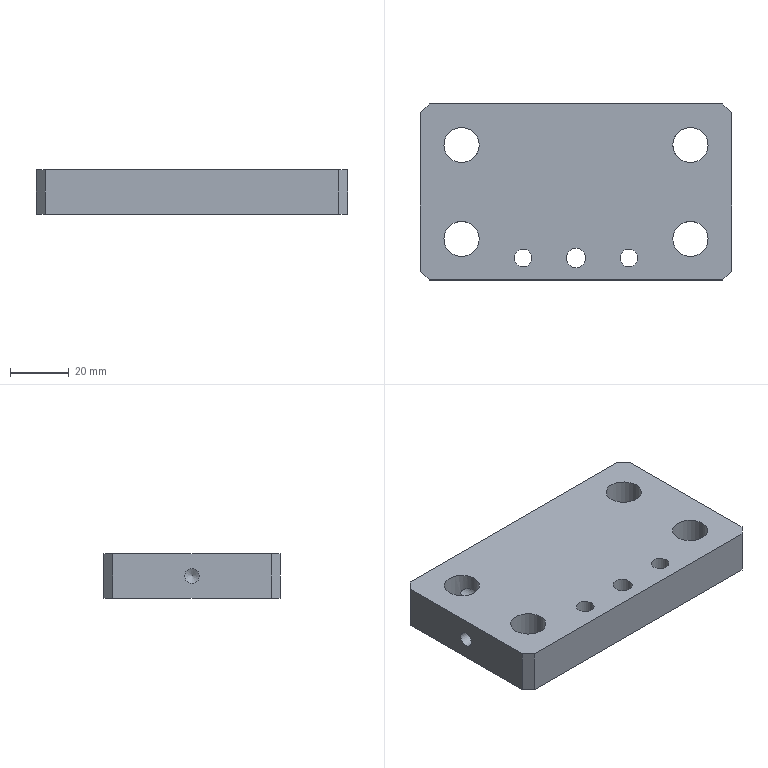Part | NX | features BREP 1 | 1 solid | 28 faces | box 106 x 60 x 15 mm | volume 85437 mm3 | cylinder 13 | plane 11 | cone 4 | commonest cylinder face diameters 5 x5 12 x4 6 x2 6.6 x1 11 x1
STEP:
#1=CARTESIAN_POINT('',(53.,0.,5.));
#2=VERTEX_POINT('',#1);
#3=CARTESIAN_POINT('',(53.,0.,7.5));
#4=DIRECTION('',(1.,0.,0.));
#5=DIRECTION('',(0.,0.,-1.));
#6=AXIS2_PLACEMENT_3D('',#3,#4,#5);
#7=CIRCLE('',#6,2.5);
#8=EDGE_CURVE('',#2,#2,#7,.T.);
#9=ORIENTED_EDGE('',*,*,#8,.F.);
#10=EDGE_LOOP('',(#9));
#11=FACE_BOUND('',#10,.T.);
#12=CARTESIAN_POINT('',(53.,-27.,0.));
#13=VERTEX_POINT('',#12);
#14=CARTESIAN_POINT('',(53.,27.,0.));
#15=VERTEX_POINT('',#14);
#16=CARTESIAN_POINT('',(53.,30.,0.));
#17=DIRECTION('',(0.,1.,0.));
#18=VECTOR('',#17,1000.);
#19=LINE('',#16,#18);
#20=EDGE_CURVE('',#13,#15,#19,.T.);
#21=ORIENTED_EDGE('',*,*,#20,.T.);
#22=CARTESIAN_POINT('',(53.,27.,15.));
#23=VERTEX_POINT('',#22);
#24=CARTESIAN_POINT('',(53.,27.,15.));
#25=DIRECTION('',(0.,0.,1.));
#26=VECTOR('',#25,1000.);
#27=LINE('',#24,#26);
#28=EDGE_CURVE('',#15,#23,#27,.T.);
#29=ORIENTED_EDGE('',*,*,#28,.T.);
#30=CARTESIAN_POINT('',(53.,-27.,15.));
#31=VERTEX_POINT('',#30);
#32=CARTESIAN_POINT('',(53.,30.,15.));
#33=DIRECTION('',(0.,1.,0.));
#34=VECTOR('',#33,1000.);
#35=LINE('',#32,#34);
#36=EDGE_CURVE('',#31,#23,#35,.T.);
#37=ORIENTED_EDGE('',*,*,#36,.F.);
#38=CARTESIAN_POINT('',(53.,-27.,15.));
#39=DIRECTION('',(0.,0.,-1.));
#40=VECTOR('',#39,1000.);
#41=LINE('',#38,#40);
#42=EDGE_CURVE('',#31,#13,#41,.T.);
#43=ORIENTED_EDGE('',*,*,#42,.T.);
#44=EDGE_LOOP('',(#21,#29,#37,#43));
#45=FACE_BOUND('',#44,.T.);
#46=CARTESIAN_POINT('',(53.,30.,15.));
#47=DIRECTION('',(-1.,0.,0.));
#48=DIRECTION('',(0.,1.,0.));
#49=AXIS2_PLACEMENT_3D('',#46,#47,#48);
#50=PLANE('',#49);
#51=ADVANCED_FACE('',(#11,#45),#50,.F.);
#52=CARTESIAN_POINT('',(32.5,30.,10.));
#53=VERTEX_POINT('',#52);
#54=CARTESIAN_POINT('',(32.5,30.,7.5));
#55=DIRECTION('',(0.,1.,0.));
#56=DIRECTION('',(0.,0.,1.));
#57=AXIS2_PLACEMENT_3D('',#54,#55,#56);
#58=CIRCLE('',#57,2.5);
#59=EDGE_CURVE('',#53,#53,#58,.T.);
#60=ORIENTED_EDGE('',*,*,#59,.F.);
#61=EDGE_LOOP('',(#60));
#62=FACE_BOUND('',#61,.T.);
#63=CARTESIAN_POINT('',(-32.5,30.,10.));
#64=VERTEX_POINT('',#63);
#65=CARTESIAN_POINT('',(-32.5,30.,7.5));
#66=DIRECTION('',(0.,1.,0.));
#67=DIRECTION('',(0.,0.,1.));
#68=AXIS2_PLACEMENT_3D('',#65,#66,#67);
#69=CIRCLE('',#68,2.5);
#70=EDGE_CURVE('',#64,#64,#69,.T.);
#71=ORIENTED_EDGE('',*,*,#70,.F.);
#72=EDGE_LOOP('',(#71));
#73=FACE_BOUND('',#72,.T.);
#74=CARTESIAN_POINT('',(50.,30.,0.));
#75=VERTEX_POINT('',#74);
#76=CARTESIAN_POINT('',(-50.,30.,0.));
#77=VERTEX_POINT('',#76);
#78=CARTESIAN_POINT('',(-53.,30.,0.));
#79=DIRECTION('',(-1.,0.,0.));
#80=VECTOR('',#79,1000.);
#81=LINE('',#78,#80);
#82=EDGE_CURVE('',#75,#77,#81,.T.);
#83=ORIENTED_EDGE('',*,*,#82,.T.);
#84=CARTESIAN_POINT('',(-50.,30.,15.));
#85=VERTEX_POINT('',#84);
#86=CARTESIAN_POINT('',(-50.,30.,15.));
#87=DIRECTION('',(0.,0.,1.));
#88=VECTOR('',#87,1000.);
#89=LINE('',#86,#88);
#90=EDGE_CURVE('',#77,#85,#89,.T.);
#91=ORIENTED_EDGE('',*,*,#90,.T.);
#92=CARTESIAN_POINT('',(50.,30.,15.));
#93=VERTEX_POINT('',#92);
#94=CARTESIAN_POINT('',(-53.,30.,15.));
#95=DIRECTION('',(-1.,0.,0.));
#96=VECTOR('',#95,1000.);
#97=LINE('',#94,#96);
#98=EDGE_CURVE('',#93,#85,#97,.T.);
#99=ORIENTED_EDGE('',*,*,#98,.F.);
#100=CARTESIAN_POINT('',(50.,30.,15.));
#101=DIRECTION('',(0.,0.,-1.));
#102=VECTOR('',#101,1000.);
#103=LINE('',#100,#102);
#104=EDGE_CURVE('',#93,#75,#103,.T.);
#105=ORIENTED_EDGE('',*,*,#104,.T.);
#106=EDGE_LOOP('',(#83,#91,#99,#105));
#107=FACE_BOUND('',#106,.T.);
#108=CARTESIAN_POINT('',(-53.,30.,15.));
#109=DIRECTION('',(0.,-1.,0.));
#110=DIRECTION('',(0.,0.,1.));
#111=AXIS2_PLACEMENT_3D('',#108,#109,#110);
#112=PLANE('',#111);
#113=ADVANCED_FACE('',(#62,#73,#107),#112,.F.);
#114=CARTESIAN_POINT('',(-53.,0.,10.));
#115=VERTEX_POINT('',#114);
#116=CARTESIAN_POINT('',(-53.,0.,7.5));
#117=DIRECTION('',(-1.,0.,0.));
#118=DIRECTION('',(0.,0.,1.));
#119=AXIS2_PLACEMENT_3D('',#116,#117,#118);
#120=CIRCLE('',#119,2.5);
#121=EDGE_CURVE('',#115,#115,#120,.T.);
#122=ORIENTED_EDGE('',*,*,#121,.F.);
#123=EDGE_LOOP('',(#122));
#124=FACE_BOUND('',#123,.T.);
#125=CARTESIAN_POINT('',(-53.,27.,15.));
#126=VERTEX_POINT('',#125);
#127=CARTESIAN_POINT('',(-53.,-27.,15.));
#128=VERTEX_POINT('',#127);
#129=CARTESIAN_POINT('',(-53.,30.,15.));
#130=DIRECTION('',(0.,-1.,0.));
#131=VECTOR('',#130,1000.);
#132=LINE('',#129,#131);
#133=EDGE_CURVE('',#126,#128,#132,.T.);
#134=ORIENTED_EDGE('',*,*,#133,.F.);
#135=CARTESIAN_POINT('',(-53.,27.,0.));
#136=VERTEX_POINT('',#135);
#137=CARTESIAN_POINT('',(-53.,27.,15.));
#138=DIRECTION('',(0.,0.,-1.));
#139=VECTOR('',#138,1000.);
#140=LINE('',#137,#139);
#141=EDGE_CURVE('',#126,#136,#140,.T.);
#142=ORIENTED_EDGE('',*,*,#141,.T.);
#143=CARTESIAN_POINT('',(-53.,-27.,0.));
#144=VERTEX_POINT('',#143);
#145=CARTESIAN_POINT('',(-53.,30.,0.));
#146=DIRECTION('',(0.,-1.,0.));
#147=VECTOR('',#146,1000.);
#148=LINE('',#145,#147);
#149=EDGE_CURVE('',#136,#144,#148,.T.);
#150=ORIENTED_EDGE('',*,*,#149,.T.);
#151=CARTESIAN_POINT('',(-53.,-27.,15.));
#152=DIRECTION('',(0.,0.,1.));
#153=VECTOR('',#152,1000.);
#154=LINE('',#151,#153);
#155=EDGE_CURVE('',#144,#128,#154,.T.);
#156=ORIENTED_EDGE('',*,*,#155,.T.);
#157=EDGE_LOOP('',(#134,#142,#150,#156));
#158=FACE_BOUND('',#157,.T.);
#159=CARTESIAN_POINT('',(-53.,30.,15.));
#160=DIRECTION('',(1.,0.,0.));
#161=DIRECTION('',(0.,-1.,0.));
#162=AXIS2_PLACEMENT_3D('',#159,#160,#161);
#163=PLANE('',#162);
#164=ADVANCED_FACE('',(#124,#158),#163,.F.);
#165=CARTESIAN_POINT('',(-50.,-30.,15.));
#166=VERTEX_POINT('',#165);
#167=CARTESIAN_POINT('',(50.,-30.,15.));
#168=VERTEX_POINT('',#167);
#169=CARTESIAN_POINT('',(-53.,-30.,15.));
#170=DIRECTION('',(1.,0.,0.));
#171=VECTOR('',#170,1000.);
#172=LINE('',#169,#171);
#173=EDGE_CURVE('',#166,#168,#172,.T.);
#174=ORIENTED_EDGE('',*,*,#173,.F.);
#175=CARTESIAN_POINT('',(-50.,-30.,0.));
#176=VERTEX_POINT('',#175);
#177=CARTESIAN_POINT('',(-50.,-30.,15.));
#178=DIRECTION('',(0.,0.,-1.));
#179=VECTOR('',#178,1000.);
#180=LINE('',#177,#179);
#181=EDGE_CURVE('',#166,#176,#180,.T.);
#182=ORIENTED_EDGE('',*,*,#181,.T.);
#183=CARTESIAN_POINT('',(50.,-30.,0.));
#184=VERTEX_POINT('',#183);
#185=CARTESIAN_POINT('',(-53.,-30.,0.));
#186=DIRECTION('',(1.,0.,0.));
#187=VECTOR('',#186,1000.);
#188=LINE('',#185,#187);
#189=EDGE_CURVE('',#176,#184,#188,.T.);
#190=ORIENTED_EDGE('',*,*,#189,.T.);
#191=CARTESIAN_POINT('',(50.,-30.,15.));
#192=DIRECTION('',(0.,0.,1.));
#193=VECTOR('',#192,1000.);
#194=LINE('',#191,#193);
#195=EDGE_CURVE('',#184,#168,#194,.T.);
#196=ORIENTED_EDGE('',*,*,#195,.T.);
#197=EDGE_LOOP('',(#174,#182,#190,#196));
#198=FACE_BOUND('',#197,.T.);
#199=CARTESIAN_POINT('',(-53.,-30.,15.));
#200=DIRECTION('',(0.,1.,0.));
#201=DIRECTION('',(0.,0.,-1.));
#202=AXIS2_PLACEMENT_3D('',#199,#200,#201);
#203=PLANE('',#202);
#204=ADVANCED_FACE('',(#198),#203,.F.);
#205=CARTESIAN_POINT('',(-3.3,-22.5,15.));
#206=VERTEX_POINT('',#205);
#207=CARTESIAN_POINT('',(0.,-22.5,15.));
#208=DIRECTION('',(0.,0.,-1.));
#209=DIRECTION('',(-1.,0.,0.));
#210=AXIS2_PLACEMENT_3D('',#207,#208,#209);
#211=CIRCLE('',#210,3.3);
#212=EDGE_CURVE('',#206,#206,#211,.T.);
#213=ORIENTED_EDGE('',*,*,#212,.T.);
#214=EDGE_LOOP('',(#213));
#215=FACE_BOUND('',#214,.T.);
#216=CARTESIAN_POINT('',(21.,-22.5,15.));
#217=VERTEX_POINT('',#216);
#218=CARTESIAN_POINT('',(18.,-22.5,15.));
#219=DIRECTION('',(0.,0.,1.));
#220=DIRECTION('',(1.,0.,0.));
#221=AXIS2_PLACEMENT_3D('',#218,#219,#220);
#222=CIRCLE('',#221,3.);
#223=EDGE_CURVE('',#217,#217,#222,.T.);
#224=ORIENTED_EDGE('',*,*,#223,.F.);
#225=EDGE_LOOP('',(#224));
#226=FACE_BOUND('',#225,.T.);
#227=CARTESIAN_POINT('',(-15.,-22.5,15.));
#228=VERTEX_POINT('',#227);
#229=CARTESIAN_POINT('',(-18.,-22.5,15.));
#230=DIRECTION('',(0.,0.,1.));
#231=DIRECTION('',(1.,0.,0.));
#232=AXIS2_PLACEMENT_3D('',#229,#230,#231);
#233=CIRCLE('',#232,3.);
#234=EDGE_CURVE('',#228,#228,#233,.T.);
#235=ORIENTED_EDGE('',*,*,#234,.F.);
#236=EDGE_LOOP('',(#235));
#237=FACE_BOUND('',#236,.T.);
#238=CARTESIAN_POINT('',(-33.,16.,15.));
#239=VERTEX_POINT('',#238);
#240=CARTESIAN_POINT('',(-39.,16.,15.));
#241=DIRECTION('',(0.,0.,1.));
#242=DIRECTION('',(1.,0.,0.));
#243=AXIS2_PLACEMENT_3D('',#240,#241,#242);
#244=CIRCLE('',#243,6.);
#245=EDGE_CURVE('',#239,#239,#244,.T.);
#246=ORIENTED_EDGE('',*,*,#245,.F.);
#247=EDGE_LOOP('',(#246));
#248=FACE_BOUND('',#247,.T.);
#249=CARTESIAN_POINT('',(-33.,-16.,15.));
#250=VERTEX_POINT('',#249);
#251=CARTESIAN_POINT('',(-39.,-16.,15.));
#252=DIRECTION('',(0.,0.,1.));
#253=DIRECTION('',(1.,0.,0.));
#254=AXIS2_PLACEMENT_3D('',#251,#252,#253);
#255=CIRCLE('',#254,6.);
#256=EDGE_CURVE('',#250,#250,#255,.T.);
#257=ORIENTED_EDGE('',*,*,#256,.F.);
#258=EDGE_LOOP('',(#257));
#259=FACE_BOUND('',#258,.T.);
#260=CARTESIAN_POINT('',(45.,16.,15.));
#261=VERTEX_POINT('',#260);
#262=CARTESIAN_POINT('',(39.,16.,15.));
#263=DIRECTION('',(0.,0.,1.));
#264=DIRECTION('',(1.,0.,0.));
#265=AXIS2_PLACEMENT_3D('',#262,#263,#264);
#266=CIRCLE('',#265,6.);
#267=EDGE_CURVE('',#261,#261,#266,.T.);
#268=ORIENTED_EDGE('',*,*,#267,.F.);
#269=EDGE_LOOP('',(#268));
#270=FACE_BOUND('',#269,.T.);
#271=CARTESIAN_POINT('',(45.,-16.,15.));
#272=VERTEX_POINT('',#271);
#273=CARTESIAN_POINT('',(39.,-16.,15.));
#274=DIRECTION('',(0.,0.,1.));
#275=DIRECTION('',(1.,0.,0.));
#276=AXIS2_PLACEMENT_3D('',#273,#274,#275);
#277=CIRCLE('',#276,6.);
#278=EDGE_CURVE('',#272,#272,#277,.T.);
#279=ORIENTED_EDGE('',*,*,#278,.F.);
#280=EDGE_LOOP('',(#279));
#281=FACE_BOUND('',#280,.T.);
#282=ORIENTED_EDGE('',*,*,#98,.T.);
#283=CARTESIAN_POINT('',(-40.,40.,15.));
#284=DIRECTION('',(-0.7071,-0.7071,0.));
#285=VECTOR('',#284,1000.);
#286=LINE('',#283,#285);
#287=EDGE_CURVE('',#85,#126,#286,.T.);
#288=ORIENTED_EDGE('',*,*,#287,.T.);
#289=ORIENTED_EDGE('',*,*,#133,.T.);
#290=CARTESIAN_POINT('',(-40.,-40.,15.));
#291=DIRECTION('',(0.7071,-0.7071,0.));
#292=VECTOR('',#291,1000.);
#293=LINE('',#290,#292);
#294=EDGE_CURVE('',#128,#166,#293,.T.);
#295=ORIENTED_EDGE('',*,*,#294,.T.);
#296=ORIENTED_EDGE('',*,*,#173,.T.);
#297=CARTESIAN_POINT('',(40.,-40.,15.));
#298=DIRECTION('',(0.7071,0.7071,0.));
#299=VECTOR('',#298,1000.);
#300=LINE('',#297,#299);
#301=EDGE_CURVE('',#168,#31,#300,.T.);
#302=ORIENTED_EDGE('',*,*,#301,.T.);
#303=ORIENTED_EDGE('',*,*,#36,.T.);
#304=CARTESIAN_POINT('',(40.,40.,15.));
#305=DIRECTION('',(-0.7071,0.7071,0.));
#306=VECTOR('',#305,1000.);
#307=LINE('',#304,#306);
#308=EDGE_CURVE('',#23,#93,#307,.T.);
#309=ORIENTED_EDGE('',*,*,#308,.T.);
#310=EDGE_LOOP('',(#282,#288,#289,#295,#296,#302,#303,#309));
#311=FACE_BOUND('',#310,.T.);
#312=CARTESIAN_POINT('',(0.,0.,15.));
#313=DIRECTION('',(0.,0.,1.));
#314=DIRECTION('',(-1.,0.,0.));
#315=AXIS2_PLACEMENT_3D('',#312,#313,#314);
#316=PLANE('',#315);
#317=ADVANCED_FACE('',(#215,#226,#237,#248,#259,#270,#281,#311),#316,.T.);
#318=CARTESIAN_POINT('',(-5.5,-22.5,0.));
#319=VERTEX_POINT('',#318);
#320=CARTESIAN_POINT('',(0.,-22.5,0.));
#321=DIRECTION('',(0.,0.,-1.));
#322=DIRECTION('',(-1.,0.,0.));
#323=AXIS2_PLACEMENT_3D('',#320,#321,#322);
#324=CIRCLE('',#323,5.5);
#325=EDGE_CURVE('',#319,#319,#324,.T.);
#326=ORIENTED_EDGE('',*,*,#325,.F.);
#327=EDGE_LOOP('',(#326));
#328=FACE_BOUND('',#327,.T.);
#329=CARTESIAN_POINT('',(21.,-22.5,0.));
#330=VERTEX_POINT('',#329);
#331=CARTESIAN_POINT('',(18.,-22.5,0.));
#332=DIRECTION('',(0.,0.,1.));
#333=DIRECTION('',(1.,0.,0.));
#334=AXIS2_PLACEMENT_3D('',#331,#332,#333);
#335=CIRCLE('',#334,3.);
#336=EDGE_CURVE('',#330,#330,#335,.T.);
#337=ORIENTED_EDGE('',*,*,#336,.T.);
#338=EDGE_LOOP('',(#337));
#339=FACE_BOUND('',#338,.T.);
#340=CARTESIAN_POINT('',(-15.,-22.5,0.));
#341=VERTEX_POINT('',#340);
#342=CARTESIAN_POINT('',(-18.,-22.5,0.));
#343=DIRECTION('',(0.,0.,1.));
#344=DIRECTION('',(1.,0.,0.));
#345=AXIS2_PLACEMENT_3D('',#342,#343,#344);
#346=CIRCLE('',#345,3.);
#347=EDGE_CURVE('',#341,#341,#346,.T.);
#348=ORIENTED_EDGE('',*,*,#347,.T.);
#349=EDGE_LOOP('',(#348));
#350=FACE_BOUND('',#349,.T.);
#351=CARTESIAN_POINT('',(-33.,16.,0.));
#352=VERTEX_POINT('',#351);
#353=CARTESIAN_POINT('',(-39.,16.,0.));
#354=DIRECTION('',(0.,0.,1.));
#355=DIRECTION('',(1.,0.,0.));
#356=AXIS2_PLACEMENT_3D('',#353,#354,#355);
#357=CIRCLE('',#356,6.);
#358=EDGE_CURVE('',#352,#352,#357,.T.);
#359=ORIENTED_EDGE('',*,*,#358,.T.);
#360=EDGE_LOOP('',(#359));
#361=FACE_BOUND('',#360,.T.);
#362=CARTESIAN_POINT('',(-33.,-16.,0.));
#363=VERTEX_POINT('',#362);
#364=CARTESIAN_POINT('',(-39.,-16.,0.));
#365=DIRECTION('',(0.,0.,1.));
#366=DIRECTION('',(1.,0.,0.));
#367=AXIS2_PLACEMENT_3D('',#364,#365,#366);
#368=CIRCLE('',#367,6.);
#369=EDGE_CURVE('',#363,#363,#368,.T.);
#370=ORIENTED_EDGE('',*,*,#369,.T.);
#371=EDGE_LOOP('',(#370));
#372=FACE_BOUND('',#371,.T.);
#373=CARTESIAN_POINT('',(45.,16.,0.));
#374=VERTEX_POINT('',#373);
#375=CARTESIAN_POINT('',(39.,16.,0.));
#376=DIRECTION('',(0.,0.,1.));
#377=DIRECTION('',(1.,0.,0.));
#378=AXIS2_PLACEMENT_3D('',#375,#376,#377);
#379=CIRCLE('',#378,6.);
#380=EDGE_CURVE('',#374,#374,#379,.T.);
#381=ORIENTED_EDGE('',*,*,#380,.T.);
#382=EDGE_LOOP('',(#381));
#383=FACE_BOUND('',#382,.T.);
#384=CARTESIAN_POINT('',(45.,-16.,0.));
#385=VERTEX_POINT('',#384);
#386=CARTESIAN_POINT('',(39.,-16.,0.));
#387=DIRECTION('',(0.,0.,1.));
#388=DIRECTION('',(1.,0.,0.));
#389=AXIS2_PLACEMENT_3D('',#386,#387,#388);
#390=CIRCLE('',#389,6.);
#391=EDGE_CURVE('',#385,#385,#390,.T.);
#392=ORIENTED_EDGE('',*,*,#391,.T.);
#393=EDGE_LOOP('',(#392));
#394=FACE_BOUND('',#393,.T.);
#395=ORIENTED_EDGE('',*,*,#149,.F.);
#396=CARTESIAN_POINT('',(-53.,27.,0.));
#397=DIRECTION('',(0.7071,0.7071,0.));
#398=VECTOR('',#397,1000.);
#399=LINE('',#396,#398);
#400=EDGE_CURVE('',#136,#77,#399,.T.);
#401=ORIENTED_EDGE('',*,*,#400,.T.);
#402=ORIENTED_EDGE('',*,*,#82,.F.);
#403=CARTESIAN_POINT('',(50.,30.,0.));
#404=DIRECTION('',(0.7071,-0.7071,0.));
#405=VECTOR('',#404,1000.);
#406=LINE('',#403,#405);
#407=EDGE_CURVE('',#75,#15,#406,.T.);
#408=ORIENTED_EDGE('',*,*,#407,.T.);
#409=ORIENTED_EDGE('',*,*,#20,.F.);
#410=CARTESIAN_POINT('',(53.,-27.,0.));
#411=DIRECTION('',(-0.7071,-0.7071,0.));
#412=VECTOR('',#411,1000.);
#413=LINE('',#410,#412);
#414=EDGE_CURVE('',#13,#184,#413,.T.);
#415=ORIENTED_EDGE('',*,*,#414,.T.);
#416=ORIENTED_EDGE('',*,*,#189,.F.);
#417=CARTESIAN_POINT('',(-50.,-30.,0.));
#418=DIRECTION('',(-0.7071,0.7071,0.));
#419=VECTOR('',#418,1000.);
#420=LINE('',#417,#419);
#421=EDGE_CURVE('',#176,#144,#420,.T.);
#422=ORIENTED_EDGE('',*,*,#421,.T.);
#423=EDGE_LOOP('',(#395,#401,#402,#408,#409,#415,#416,#422));
#424=FACE_BOUND('',#423,.T.);
#425=CARTESIAN_POINT('',(0.,0.,0.));
#426=DIRECTION('',(0.,0.,1.));
#427=DIRECTION('',(-1.,0.,0.));
#428=AXIS2_PLACEMENT_3D('',#425,#426,#427);
#429=PLANE('',#428);
#430=ADVANCED_FACE('',(#328,#339,#350,#361,#372,#383,#394,#424),#429,.F.);
#431=ORIENTED_EDGE('',*,*,#391,.F.);
#432=EDGE_LOOP('',(#431));
#433=FACE_BOUND('',#432,.T.);
#434=ORIENTED_EDGE('',*,*,#278,.T.);
#435=EDGE_LOOP('',(#434));
#436=FACE_BOUND('',#435,.T.);
#437=CARTESIAN_POINT('',(39.,-16.,15.));
#438=DIRECTION('',(0.,0.,1.));
#439=DIRECTION('',(-1.,0.,0.));
#440=AXIS2_PLACEMENT_3D('',#437,#438,#439);
#441=CYLINDRICAL_SURFACE('',#440,6.);
#442=ADVANCED_FACE('',(#433,#436),#441,.F.);
#443=CARTESIAN_POINT('',(33.084,15.,5.069));
#444=VERTEX_POINT('',#443);
#445=CARTESIAN_POINT('',(33.084,15.,9.931));
#446=VERTEX_POINT('',#445);
#447=CARTESIAN_POINT('',(33.084,15.,5.069));
#448=CARTESIAN_POINT('',(33.121,14.78,5.455));
#449=CARTESIAN_POINT('',(33.219,14.353,6.213));
#450=CARTESIAN_POINT('',(33.404,13.829,7.503));
#451=CARTESIAN_POINT('',(33.218,14.355,8.789));
#452=CARTESIAN_POINT('',(33.121,14.781,9.546));
#453=CARTESIAN_POINT('',(33.084,15.,9.931));
#454=B_SPLINE_CURVE_WITH_KNOTS('',3,(#447,#448,#449,#450,#451,#452,#453),.UNSPECIFIED.,.F.,.F.,(4,1,1,1,4),(0.,0.001335,0.002669,0.004004,0.005339),.UNSPECIFIED.);
#455=EDGE_CURVE('',#444,#446,#454,.T.);
#456=ORIENTED_EDGE('',*,*,#455,.T.);
#457=CARTESIAN_POINT('',(33.084,15.,9.931));
#458=CARTESIAN_POINT('',(32.983,15.598,9.955));
#459=CARTESIAN_POINT('',(32.966,16.805,9.957));
#460=CARTESIAN_POINT('',(33.461,18.547,9.846));
#461=CARTESIAN_POINT('',(34.481,20.042,9.275));
#462=CARTESIAN_POINT('',(35.257,20.685,7.513));
#463=CARTESIAN_POINT('',(34.492,20.053,5.735));
#464=CARTESIAN_POINT('',(33.471,18.568,5.157));
#465=CARTESIAN_POINT('',(32.966,16.82,5.043));
#466=CARTESIAN_POINT('',(32.983,15.598,5.045));
#467=CARTESIAN_POINT('',(33.084,15.,5.069));
#468=B_SPLINE_CURVE_WITH_KNOTS('',3,(#457,#458,#459,#460,#461,#462,#463,#464,#465,#466,#467),.UNSPECIFIED.,.F.,.F.,(4,1,1,1,1,1,1,1,4),(0.,0.001794,0.003588,0.005381,0.007175,0.008969,0.01076,0.01256,0.01435),.UNSPECIFIED.);
#469=EDGE_CURVE('',#446,#444,#468,.T.);
#470=ORIENTED_EDGE('',*,*,#469,.T.);
#471=EDGE_LOOP('',(#456,#470));
#472=FACE_BOUND('',#471,.T.);
#473=ORIENTED_EDGE('',*,*,#380,.F.);
#474=EDGE_LOOP('',(#473));
#475=FACE_BOUND('',#474,.T.);
#476=ORIENTED_EDGE('',*,*,#267,.T.);
#477=EDGE_LOOP('',(#476));
#478=FACE_BOUND('',#477,.T.);
#479=CARTESIAN_POINT('',(39.,16.,15.));
#480=DIRECTION('',(0.,0.,1.));
#481=DIRECTION('',(-1.,0.,0.));
#482=AXIS2_PLACEMENT_3D('',#479,#480,#481);
#483=CYLINDRICAL_SURFACE('',#482,6.);
#484=ADVANCED_FACE('',(#472,#475,#478),#483,.F.);
#485=ORIENTED_EDGE('',*,*,#369,.F.);
#486=EDGE_LOOP('',(#485));
#487=FACE_BOUND('',#486,.T.);
#488=ORIENTED_EDGE('',*,*,#256,.T.);
#489=EDGE_LOOP('',(#488));
#490=FACE_BOUND('',#489,.T.);
#491=CARTESIAN_POINT('',(-39.,-16.,15.));
#492=DIRECTION('',(0.,0.,1.));
#493=DIRECTION('',(-1.,0.,0.));
#494=AXIS2_PLACEMENT_3D('',#491,#492,#493);
#495=CYLINDRICAL_SURFACE('',#494,6.);
#496=ADVANCED_FACE('',(#487,#490),#495,.F.);
#497=CARTESIAN_POINT('',(-33.084,15.,9.931));
#498=VERTEX_POINT('',#497);
#499=CARTESIAN_POINT('',(-33.084,15.,5.069));
#500=VERTEX_POINT('',#499);
#501=CARTESIAN_POINT('',(-33.084,15.,9.931));
#502=CARTESIAN_POINT('',(-33.121,14.78,9.545));
#503=CARTESIAN_POINT('',(-33.219,14.353,8.787));
#504=CARTESIAN_POINT('',(-33.404,13.829,7.497));
#505=CARTESIAN_POINT('',(-33.218,14.355,6.211));
#506=CARTESIAN_POINT('',(-33.121,14.781,5.454));
#507=CARTESIAN_POINT('',(-33.084,15.,5.069));
#508=B_SPLINE_CURVE_WITH_KNOTS('',3,(#501,#502,#503,#504,#505,#506,#507),.UNSPECIFIED.,.F.,.F.,(4,1,1,1,4),(0.,0.001335,0.002669,0.004004,0.005339),.UNSPECIFIED.);
#509=EDGE_CURVE('',#498,#500,#508,.T.);
#510=ORIENTED_EDGE('',*,*,#509,.T.);
#511=CARTESIAN_POINT('',(-33.084,15.,5.069));
#512=CARTESIAN_POINT('',(-32.983,15.598,5.045));
#513=CARTESIAN_POINT('',(-32.966,16.805,5.043));
#514=CARTESIAN_POINT('',(-33.461,18.547,5.154));
#515=CARTESIAN_POINT('',(-34.481,20.042,5.725));
#516=CARTESIAN_POINT('',(-35.257,20.685,7.487));
#517=CARTESIAN_POINT('',(-34.492,20.053,9.265));
#518=CARTESIAN_POINT('',(-33.471,18.568,9.843));
#519=CARTESIAN_POINT('',(-32.966,16.82,9.957));
#520=CARTESIAN_POINT('',(-32.983,15.598,9.955));
#521=CARTESIAN_POINT('',(-33.084,15.,9.931));
#522=B_SPLINE_CURVE_WITH_KNOTS('',3,(#511,#512,#513,#514,#515,#516,#517,#518,#519,#520,#521),.UNSPECIFIED.,.F.,.F.,(4,1,1,1,1,1,1,1,4),(0.,0.001794,0.003588,0.005381,0.007175,0.008969,0.01076,0.01256,0.01435),.UNSPECIFIED.);
#523=EDGE_CURVE('',#500,#498,#522,.T.);
#524=ORIENTED_EDGE('',*,*,#523,.T.);
#525=EDGE_LOOP('',(#510,#524));
#526=FACE_BOUND('',#525,.T.);
#527=ORIENTED_EDGE('',*,*,#358,.F.);
#528=EDGE_LOOP('',(#527));
#529=FACE_BOUND('',#528,.T.);
#530=ORIENTED_EDGE('',*,*,#245,.T.);
#531=EDGE_LOOP('',(#530));
#532=FACE_BOUND('',#531,.T.);
#533=CARTESIAN_POINT('',(-39.,16.,15.));
#534=DIRECTION('',(0.,0.,1.));
#535=DIRECTION('',(-1.,0.,0.));
#536=AXIS2_PLACEMENT_3D('',#533,#534,#535);
#537=CYLINDRICAL_SURFACE('',#536,6.);
#538=ADVANCED_FACE('',(#526,#529,#532),#537,.F.);
#539=ORIENTED_EDGE('',*,*,#287,.F.);
#540=ORIENTED_EDGE('',*,*,#90,.F.);
#541=ORIENTED_EDGE('',*,*,#400,.F.);
#542=ORIENTED_EDGE('',*,*,#141,.F.);
#543=EDGE_LOOP('',(#539,#540,#541,#542));
#544=FACE_BOUND('',#543,.T.);
#545=CARTESIAN_POINT('',(-53.,27.,15.));
#546=DIRECTION('',(0.7071,-0.7071,0.));
#547=DIRECTION('',(0.,0.,1.));
#548=AXIS2_PLACEMENT_3D('',#545,#546,#547);
#549=PLANE('',#548);
#550=ADVANCED_FACE('',(#544),#549,.F.);
#551=ORIENTED_EDGE('',*,*,#294,.F.);
#552=ORIENTED_EDGE('',*,*,#155,.F.);
#553=ORIENTED_EDGE('',*,*,#421,.F.);
#554=ORIENTED_EDGE('',*,*,#181,.F.);
#555=EDGE_LOOP('',(#551,#552,#553,#554));
#556=FACE_BOUND('',#555,.T.);
#557=CARTESIAN_POINT('',(-50.,-30.,15.));
#558=DIRECTION('',(0.7071,0.7071,0.));
#559=DIRECTION('',(0.,0.,1.));
#560=AXIS2_PLACEMENT_3D('',#557,#558,#559);
#561=PLANE('',#560);
#562=ADVANCED_FACE('',(#556),#561,.F.);
#563=ORIENTED_EDGE('',*,*,#308,.F.);
#564=ORIENTED_EDGE('',*,*,#28,.F.);
#565=ORIENTED_EDGE('',*,*,#407,.F.);
#566=ORIENTED_EDGE('',*,*,#104,.F.);
#567=EDGE_LOOP('',(#563,#564,#565,#566));
#568=FACE_BOUND('',#567,.T.);
#569=CARTESIAN_POINT('',(50.,30.,15.));
#570=DIRECTION('',(-0.7071,-0.7071,0.));
#571=DIRECTION('',(0.,0.,1.));
#572=AXIS2_PLACEMENT_3D('',#569,#570,#571);
#573=PLANE('',#572);
#574=ADVANCED_FACE('',(#568),#573,.F.);
#575=ORIENTED_EDGE('',*,*,#301,.F.);
#576=ORIENTED_EDGE('',*,*,#195,.F.);
#577=ORIENTED_EDGE('',*,*,#414,.F.);
#578=ORIENTED_EDGE('',*,*,#42,.F.);
#579=EDGE_LOOP('',(#575,#576,#577,#578));
#580=FACE_BOUND('',#579,.T.);
#581=CARTESIAN_POINT('',(53.,-27.,15.));
#582=DIRECTION('',(-0.7071,0.7071,0.));
#583=DIRECTION('',(0.,0.,1.));
#584=AXIS2_PLACEMENT_3D('',#581,#582,#583);
#585=PLANE('',#584);
#586=ADVANCED_FACE('',(#580),#585,.F.);
#587=ORIENTED_EDGE('',*,*,#347,.F.);
#588=EDGE_LOOP('',(#587));
#589=FACE_BOUND('',#588,.T.);
#590=ORIENTED_EDGE('',*,*,#234,.T.);
#591=EDGE_LOOP('',(#590));
#592=FACE_BOUND('',#591,.T.);
#593=CARTESIAN_POINT('',(-18.,-22.5,15.));
#594=DIRECTION('',(0.,0.,1.));
#595=DIRECTION('',(-1.,0.,0.));
#596=AXIS2_PLACEMENT_3D('',#593,#594,#595);
#597=CYLINDRICAL_SURFACE('',#596,3.);
#598=ADVANCED_FACE('',(#589,#592),#597,.F.);
#599=ORIENTED_EDGE('',*,*,#336,.F.);
#600=EDGE_LOOP('',(#599));
#601=FACE_BOUND('',#600,.T.);
#602=ORIENTED_EDGE('',*,*,#223,.T.);
#603=EDGE_LOOP('',(#602));
#604=FACE_BOUND('',#603,.T.);
#605=CARTESIAN_POINT('',(18.,-22.5,15.));
#606=DIRECTION('',(0.,0.,1.));
#607=DIRECTION('',(-1.,0.,0.));
#608=AXIS2_PLACEMENT_3D('',#605,#606,#607);
#609=CYLINDRICAL_SURFACE('',#608,3.);
#610=ADVANCED_FACE('',(#601,#604),#609,.F.);
#611=ORIENTED_EDGE('',*,*,#212,.F.);
#612=EDGE_LOOP('',(#611));
#613=FACE_BOUND('',#612,.T.);
#614=CARTESIAN_POINT('',(-3.3,-22.5,6.4));
#615=VERTEX_POINT('',#614);
#616=CARTESIAN_POINT('',(0.,-22.5,6.4));
#617=DIRECTION('',(0.,0.,-1.));
#618=DIRECTION('',(-1.,0.,0.));
#619=AXIS2_PLACEMENT_3D('',#616,#617,#618);
#620=CIRCLE('',#619,3.3);
#621=EDGE_CURVE('',#615,#615,#620,.T.);
#622=ORIENTED_EDGE('',*,*,#621,.T.);
#623=EDGE_LOOP('',(#622));
#624=FACE_BOUND('',#623,.T.);
#625=CARTESIAN_POINT('',(0.,-22.5,0.));
#626=DIRECTION('',(0.,0.,-1.));
#627=DIRECTION('',(1.,0.,0.));
#628=AXIS2_PLACEMENT_3D('',#625,#626,#627);
#629=CYLINDRICAL_SURFACE('',#628,3.3);
#630=ADVANCED_FACE('',(#613,#624),#629,.F.);
#631=ORIENTED_EDGE('',*,*,#621,.F.);
#632=EDGE_LOOP('',(#631));
#633=FACE_BOUND('',#632,.T.);
#634=CARTESIAN_POINT('',(-5.5,-22.5,6.4));
#635=VERTEX_POINT('',#634);
#636=CARTESIAN_POINT('',(0.,-22.5,6.4));
#637=DIRECTION('',(0.,0.,-1.));
#638=DIRECTION('',(-1.,0.,0.));
#639=AXIS2_PLACEMENT_3D('',#636,#637,#638);
#640=CIRCLE('',#639,5.5);
#641=EDGE_CURVE('',#635,#635,#640,.T.);
#642=ORIENTED_EDGE('',*,*,#641,.T.);
#643=EDGE_LOOP('',(#642));
#644=FACE_BOUND('',#643,.T.);
#645=CARTESIAN_POINT('',(3.3,-22.5,6.4));
#646=DIRECTION('',(0.,0.,1.));
#647=DIRECTION('',(-1.,0.,0.));
#648=AXIS2_PLACEMENT_3D('',#645,#646,#647);
#649=PLANE('',#648);
#650=ADVANCED_FACE('',(#633,#644),#649,.F.);
#651=ORIENTED_EDGE('',*,*,#641,.F.);
#652=EDGE_LOOP('',(#651));
#653=FACE_BOUND('',#652,.T.);
#654=ORIENTED_EDGE('',*,*,#325,.T.);
#655=EDGE_LOOP('',(#654));
#656=FACE_BOUND('',#655,.T.);
#657=CARTESIAN_POINT('',(0.,-22.5,0.));
#658=DIRECTION('',(0.,0.,-1.));
#659=DIRECTION('',(1.,0.,0.));
#660=AXIS2_PLACEMENT_3D('',#657,#658,#659);
#661=CYLINDRICAL_SURFACE('',#660,5.5);
#662=ADVANCED_FACE('',(#653,#656),#661,.F.);
#663=CARTESIAN_POINT('',(-36.498,0.,7.5));
#664=VERTEX_POINT('',#663);
#665=VERTEX_LOOP('',#664);
#666=FACE_BOUND('',#665,.T.);
#667=CARTESIAN_POINT('',(-38.,0.,10.));
#668=VERTEX_POINT('',#667);
#669=CARTESIAN_POINT('',(-38.,0.,7.5));
#670=DIRECTION('',(-1.,0.,0.));
#671=DIRECTION('',(0.,0.,1.));
#672=AXIS2_PLACEMENT_3D('',#669,#670,#671);
#673=CIRCLE('',#672,2.5);
#674=EDGE_CURVE('',#668,#668,#673,.T.);
#675=ORIENTED_EDGE('',*,*,#674,.T.);
#676=EDGE_LOOP('',(#675));
#677=FACE_BOUND('',#676,.T.);
#678=CARTESIAN_POINT('',(-38.,0.,7.5));
#679=DIRECTION('',(-1.,0.,0.));
#680=DIRECTION('',(0.,0.,-1.));
#681=AXIS2_PLACEMENT_3D('',#678,#679,#680);
#682=CONICAL_SURFACE('',#681,2.5,1.03);
#683=ADVANCED_FACE('',(#666,#677),#682,.F.);
#684=ORIENTED_EDGE('',*,*,#674,.F.);
#685=EDGE_LOOP('',(#684));
#686=FACE_BOUND('',#685,.T.);
#687=ORIENTED_EDGE('',*,*,#121,.T.);
#688=EDGE_LOOP('',(#687));
#689=FACE_BOUND('',#688,.T.);
#690=CARTESIAN_POINT('',(-53.,0.,7.5));
#691=DIRECTION('',(-1.,0.,0.));
#692=DIRECTION('',(0.,0.,-1.));
#693=AXIS2_PLACEMENT_3D('',#690,#691,#692);
#694=CYLINDRICAL_SURFACE('',#693,2.5);
#695=ADVANCED_FACE('',(#686,#689),#694,.F.);
#696=ORIENTED_EDGE('',*,*,#70,.T.);
#697=EDGE_LOOP('',(#696));
#698=FACE_BOUND('',#697,.T.);
#699=CARTESIAN_POINT('',(-32.5,15.,7.5));
#700=DIRECTION('',(0.,1.,0.));
#701=DIRECTION('',(0.,0.,1.));
#702=AXIS2_PLACEMENT_3D('',#699,#700,#701);
#703=CIRCLE('',#702,2.5);
#704=EDGE_CURVE('',#498,#500,#703,.T.);
#705=ORIENTED_EDGE('',*,*,#704,.F.);
#706=ORIENTED_EDGE('',*,*,#523,.F.);
#707=EDGE_LOOP('',(#705,#706));
#708=FACE_BOUND('',#707,.T.);
#709=CARTESIAN_POINT('',(-32.5,30.,7.5));
#710=DIRECTION('',(0.,1.,0.));
#711=DIRECTION('',(0.,0.,-1.));
#712=AXIS2_PLACEMENT_3D('',#709,#710,#711);
#713=CYLINDRICAL_SURFACE('',#712,2.5);
#714=ADVANCED_FACE('',(#698,#708),#713,.F.);
#715=ORIENTED_EDGE('',*,*,#704,.T.);
#716=ORIENTED_EDGE('',*,*,#509,.F.);
#717=EDGE_LOOP('',(#715,#716));
#718=FACE_BOUND('',#717,.T.);
#719=CARTESIAN_POINT('',(-32.5,15.,7.5));
#720=DIRECTION('',(0.,1.,0.));
#721=DIRECTION('',(0.,0.,-1.));
#722=AXIS2_PLACEMENT_3D('',#719,#720,#721);
#723=CONICAL_SURFACE('',#722,2.5,1.03);
#724=ADVANCED_FACE('',(#718),#723,.F.);
#725=ORIENTED_EDGE('',*,*,#59,.T.);
#726=EDGE_LOOP('',(#725));
#727=FACE_BOUND('',#726,.T.);
#728=CARTESIAN_POINT('',(32.5,15.,7.5));
#729=DIRECTION('',(0.,1.,0.));
#730=DIRECTION('',(0.,0.,1.));
#731=AXIS2_PLACEMENT_3D('',#728,#729,#730);
#732=CIRCLE('',#731,2.5);
#733=EDGE_CURVE('',#444,#446,#732,.T.);
#734=ORIENTED_EDGE('',*,*,#733,.F.);
#735=ORIENTED_EDGE('',*,*,#469,.F.);
#736=EDGE_LOOP('',(#734,#735));
#737=FACE_BOUND('',#736,.T.);
#738=CARTESIAN_POINT('',(32.5,30.,7.5));
#739=DIRECTION('',(0.,1.,0.));
#740=DIRECTION('',(0.,0.,-1.));
#741=AXIS2_PLACEMENT_3D('',#738,#739,#740);
#742=CYLINDRICAL_SURFACE('',#741,2.5);
#743=ADVANCED_FACE('',(#727,#737),#742,.F.);
#744=ORIENTED_EDGE('',*,*,#733,.T.);
#745=ORIENTED_EDGE('',*,*,#455,.F.);
#746=EDGE_LOOP('',(#744,#745));
#747=FACE_BOUND('',#746,.T.);
#748=CARTESIAN_POINT('',(32.5,15.,7.5));
#749=DIRECTION('',(0.,1.,0.));
#750=DIRECTION('',(0.,0.,-1.));
#751=AXIS2_PLACEMENT_3D('',#748,#749,#750);
#752=CONICAL_SURFACE('',#751,2.5,1.03);
#753=ADVANCED_FACE('',(#747),#752,.F.);
#754=CARTESIAN_POINT('',(36.498,0.,7.5));
#755=VERTEX_POINT('',#754);
#756=VERTEX_LOOP('',#755);
#757=FACE_BOUND('',#756,.T.);
#758=CARTESIAN_POINT('',(38.,0.,5.));
#759=VERTEX_POINT('',#758);
#760=CARTESIAN_POINT('',(38.,0.,7.5));
#761=DIRECTION('',(1.,0.,0.));
#762=DIRECTION('',(0.,0.,-1.));
#763=AXIS2_PLACEMENT_3D('',#760,#761,#762);
#764=CIRCLE('',#763,2.5);
#765=EDGE_CURVE('',#759,#759,#764,.T.);
#766=ORIENTED_EDGE('',*,*,#765,.T.);
#767=EDGE_LOOP('',(#766));
#768=FACE_BOUND('',#767,.T.);
#769=CARTESIAN_POINT('',(38.,0.,7.5));
#770=DIRECTION('',(1.,0.,0.));
#771=DIRECTION('',(0.,0.,1.));
#772=AXIS2_PLACEMENT_3D('',#769,#770,#771);
#773=CONICAL_SURFACE('',#772,2.5,1.03);
#774=ADVANCED_FACE('',(#757,#768),#773,.F.);
#775=ORIENTED_EDGE('',*,*,#765,.F.);
#776=EDGE_LOOP('',(#775));
#777=FACE_BOUND('',#776,.T.);
#778=ORIENTED_EDGE('',*,*,#8,.T.);
#779=EDGE_LOOP('',(#778));
#780=FACE_BOUND('',#779,.T.);
#781=CARTESIAN_POINT('',(53.,0.,7.5));
#782=DIRECTION('',(1.,0.,0.));
#783=DIRECTION('',(0.,0.,1.));
#784=AXIS2_PLACEMENT_3D('',#781,#782,#783);
#785=CYLINDRICAL_SURFACE('',#784,2.5);
#786=ADVANCED_FACE('',(#777,#780),#785,.F.);
#787=CLOSED_SHELL('',(#51,#113,#164,#204,#317,#430,#442,#484,#496,#538,#550,#562,#574,#586,#598,#610,#630,#650,#662,#683,#695,#714,#724,#743,#753,#774,#786));
#788=MANIFOLD_SOLID_BREP('',#787);
#789=(LENGTH_UNIT()NAMED_UNIT(*)SI_UNIT(.MILLI.,.METRE.));
#790=UNCERTAINTY_MEASURE_WITH_UNIT(LENGTH_MEASURE(0.0508),#789,'','');
#791=(NAMED_UNIT(*)PLANE_ANGLE_UNIT()SI_UNIT($,.RADIAN.));
#792=(NAMED_UNIT(*)SI_UNIT($,.STERADIAN.)SOLID_ANGLE_UNIT());
#793=(GEOMETRIC_REPRESENTATION_CONTEXT(3)GLOBAL_UNCERTAINTY_ASSIGNED_CONTEXT((#790))GLOBAL_UNIT_ASSIGNED_CONTEXT((#789,#791,#792))REPRESENTATION_CONTEXT('',''));
#794=ADVANCED_BREP_SHAPE_REPRESENTATION('',(#788),#793);